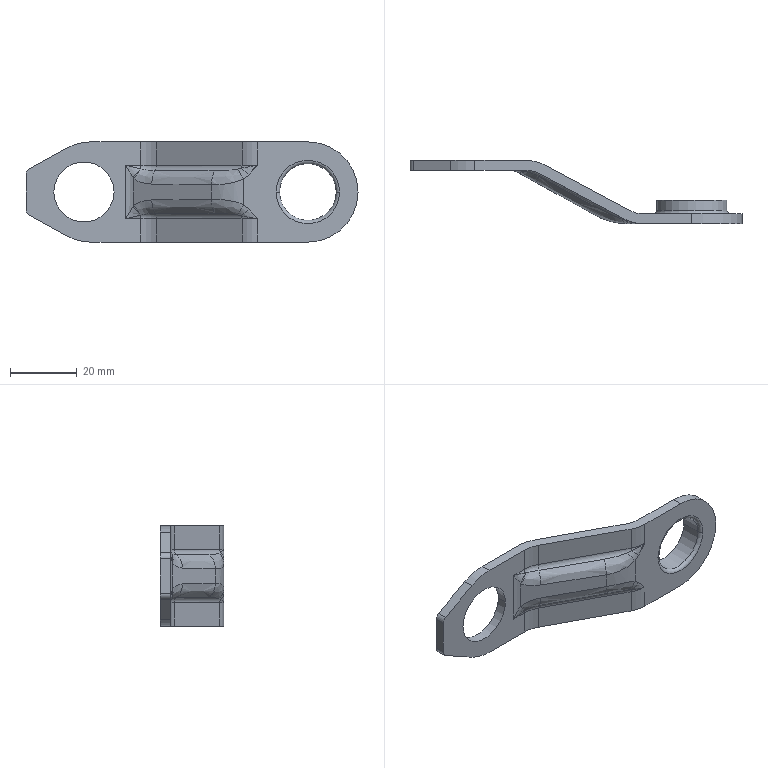Part | NX | features BREP 1 | 1 solid | 87 faces | box 99.333 x 19 x 30 mm | volume 7801 mm3 | cylinder 31 | spline 28 | plane 16 | torus 12 | commonest cylinder face diameters 4 x6 10 x5 20 x4 30 x3 14 x2 17 x2